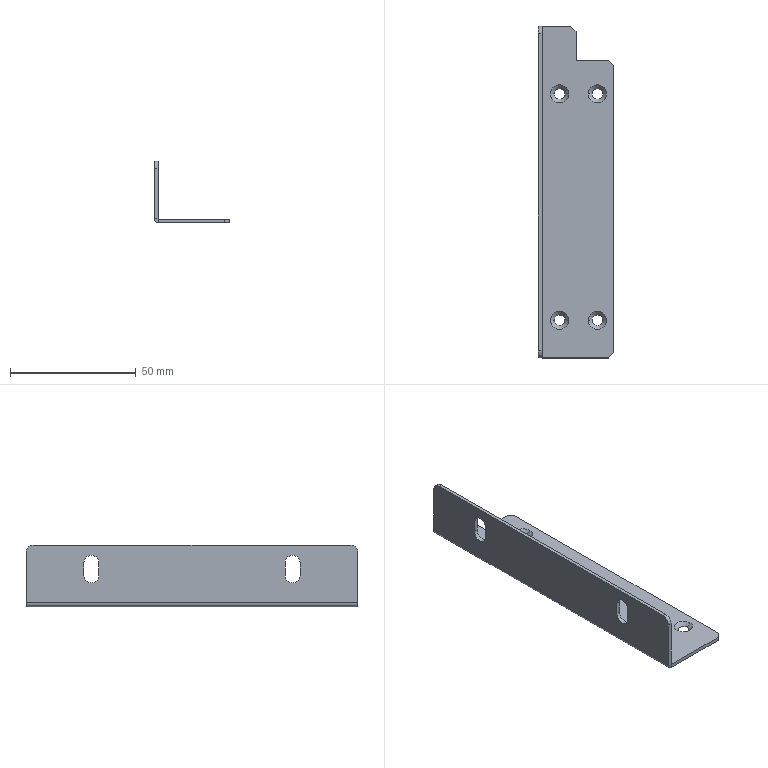Part | SolidWorks | features ICE 3, CornerTrim 2, Chamfer 1, EdgeFlange 1, FlatPattern 1, SMBaseFlange 1, SheetMetal 1 | 1 solid | 39 faces | box 30 x 132 x 24.5 mm | volume 9772 mm3 | plane 21 | cylinder 10 | cone 8 | commonest cylinder face diameters 6 x8 0.2 x1 3.2 x1
STEP:
#1=CARTESIAN_POINT('',(-8.6,39.,-1.5));
#2=VERTEX_POINT('',#1);
#3=CARTESIAN_POINT('',(-4.4,39.,-1.5));
#4=VERTEX_POINT('',#3);
#5=CARTESIAN_POINT('',(-6.5,39.,-1.5));
#6=DIRECTION('',(0.,0.,1.));
#7=DIRECTION('',(1.,0.,0.));
#8=AXIS2_PLACEMENT_3D('',#5,#6,#7);
#9=CIRCLE('',#8,2.1);
#10=EDGE_CURVE('',#2,#4,#9,.T.);
#11=ORIENTED_EDGE('',*,*,#10,.F.);
#12=CARTESIAN_POINT('',(-10.1,39.,0.));
#13=VERTEX_POINT('',#12);
#14=CARTESIAN_POINT('',(-8.6,39.,-1.5));
#15=DIRECTION('',(-0.7071,0.,0.7071));
#16=VECTOR('',#15,1000.);
#17=LINE('',#14,#16);
#18=EDGE_CURVE('',#2,#13,#17,.T.);
#19=ORIENTED_EDGE('',*,*,#18,.T.);
#20=CARTESIAN_POINT('',(-2.9,39.,0.));
#21=VERTEX_POINT('',#20);
#22=CARTESIAN_POINT('',(-6.5,39.,0.));
#23=DIRECTION('',(0.,0.,-1.));
#24=DIRECTION('',(1.,0.,0.));
#25=AXIS2_PLACEMENT_3D('',#22,#23,#24);
#26=CIRCLE('',#25,3.6);
#27=EDGE_CURVE('',#21,#13,#26,.T.);
#28=ORIENTED_EDGE('',*,*,#27,.F.);
#29=CARTESIAN_POINT('',(-4.4,39.,-1.5));
#30=DIRECTION('',(0.7071,0.,0.7071));
#31=VECTOR('',#30,1000.);
#32=LINE('',#29,#31);
#33=EDGE_CURVE('',#4,#21,#32,.T.);
#34=ORIENTED_EDGE('',*,*,#33,.F.);
#35=EDGE_LOOP('',(#11,#19,#28,#34));
#36=FACE_OUTER_BOUND('',#35,.T.);
#37=CARTESIAN_POINT('',(-6.5,39.,-1.5));
#38=DIRECTION('',(0.,0.,1.));
#39=DIRECTION('',(1.,0.,0.));
#40=AXIS2_PLACEMENT_3D('',#37,#38,#39);
#41=CONICAL_SURFACE('',#40,2.1,0.7854);
#42=ADVANCED_FACE('',(#36),#41,.F.);
#43=CARTESIAN_POINT('',(6.4,39.,-1.5));
#44=VERTEX_POINT('',#43);
#45=CARTESIAN_POINT('',(10.6,39.,-1.5));
#46=VERTEX_POINT('',#45);
#47=CARTESIAN_POINT('',(8.5,39.,-1.5));
#48=DIRECTION('',(0.,0.,1.));
#49=DIRECTION('',(1.,0.,0.));
#50=AXIS2_PLACEMENT_3D('',#47,#48,#49);
#51=CIRCLE('',#50,2.1);
#52=EDGE_CURVE('',#44,#46,#51,.T.);
#53=ORIENTED_EDGE('',*,*,#52,.F.);
#54=CARTESIAN_POINT('',(4.9,39.,0.));
#55=VERTEX_POINT('',#54);
#56=CARTESIAN_POINT('',(6.4,39.,-1.5));
#57=DIRECTION('',(-0.7071,0.,0.7071));
#58=VECTOR('',#57,1000.);
#59=LINE('',#56,#58);
#60=EDGE_CURVE('',#44,#55,#59,.T.);
#61=ORIENTED_EDGE('',*,*,#60,.T.);
#62=CARTESIAN_POINT('',(12.1,39.,0.));
#63=VERTEX_POINT('',#62);
#64=CARTESIAN_POINT('',(8.5,39.,0.));
#65=DIRECTION('',(0.,0.,-1.));
#66=DIRECTION('',(1.,0.,0.));
#67=AXIS2_PLACEMENT_3D('',#64,#65,#66);
#68=CIRCLE('',#67,3.6);
#69=EDGE_CURVE('',#63,#55,#68,.T.);
#70=ORIENTED_EDGE('',*,*,#69,.F.);
#71=CARTESIAN_POINT('',(10.6,39.,-1.5));
#72=DIRECTION('',(0.7071,0.,0.7071));
#73=VECTOR('',#72,1000.);
#74=LINE('',#71,#73);
#75=EDGE_CURVE('',#46,#63,#74,.T.);
#76=ORIENTED_EDGE('',*,*,#75,.F.);
#77=EDGE_LOOP('',(#53,#61,#70,#76));
#78=FACE_OUTER_BOUND('',#77,.T.);
#79=CARTESIAN_POINT('',(8.5,39.,-1.5));
#80=DIRECTION('',(0.,0.,1.));
#81=DIRECTION('',(1.,0.,0.));
#82=AXIS2_PLACEMENT_3D('',#79,#80,#81);
#83=CONICAL_SURFACE('',#82,2.1,0.7854);
#84=ADVANCED_FACE('',(#78),#83,.F.);
#85=CARTESIAN_POINT('',(6.4,-51.,-1.5));
#86=VERTEX_POINT('',#85);
#87=CARTESIAN_POINT('',(10.6,-51.,-1.5));
#88=VERTEX_POINT('',#87);
#89=CARTESIAN_POINT('',(8.5,-51.,-1.5));
#90=DIRECTION('',(0.,0.,1.));
#91=DIRECTION('',(1.,0.,0.));
#92=AXIS2_PLACEMENT_3D('',#89,#90,#91);
#93=CIRCLE('',#92,2.1);
#94=EDGE_CURVE('',#86,#88,#93,.T.);
#95=ORIENTED_EDGE('',*,*,#94,.F.);
#96=CARTESIAN_POINT('',(4.9,-51.,0.));
#97=VERTEX_POINT('',#96);
#98=CARTESIAN_POINT('',(6.4,-51.,-1.5));
#99=DIRECTION('',(-0.7071,0.,0.7071));
#100=VECTOR('',#99,1000.);
#101=LINE('',#98,#100);
#102=EDGE_CURVE('',#86,#97,#101,.T.);
#103=ORIENTED_EDGE('',*,*,#102,.T.);
#104=CARTESIAN_POINT('',(12.1,-51.,0.));
#105=VERTEX_POINT('',#104);
#106=CARTESIAN_POINT('',(8.5,-51.,0.));
#107=DIRECTION('',(0.,0.,-1.));
#108=DIRECTION('',(1.,0.,0.));
#109=AXIS2_PLACEMENT_3D('',#106,#107,#108);
#110=CIRCLE('',#109,3.6);
#111=EDGE_CURVE('',#105,#97,#110,.T.);
#112=ORIENTED_EDGE('',*,*,#111,.F.);
#113=CARTESIAN_POINT('',(10.6,-51.,-1.5));
#114=DIRECTION('',(0.7071,0.,0.7071));
#115=VECTOR('',#114,1000.);
#116=LINE('',#113,#115);
#117=EDGE_CURVE('',#88,#105,#116,.T.);
#118=ORIENTED_EDGE('',*,*,#117,.F.);
#119=EDGE_LOOP('',(#95,#103,#112,#118));
#120=FACE_OUTER_BOUND('',#119,.T.);
#121=CARTESIAN_POINT('',(8.5,-51.,-1.5));
#122=DIRECTION('',(0.,0.,1.));
#123=DIRECTION('',(1.,0.,0.));
#124=AXIS2_PLACEMENT_3D('',#121,#122,#123);
#125=CONICAL_SURFACE('',#124,2.1,0.7854);
#126=ADVANCED_FACE('',(#120),#125,.F.);
#127=CARTESIAN_POINT('',(-8.6,-51.,-1.5));
#128=VERTEX_POINT('',#127);
#129=CARTESIAN_POINT('',(-4.4,-51.,-1.5));
#130=VERTEX_POINT('',#129);
#131=CARTESIAN_POINT('',(-6.5,-51.,-1.5));
#132=DIRECTION('',(0.,0.,1.));
#133=DIRECTION('',(1.,0.,0.));
#134=AXIS2_PLACEMENT_3D('',#131,#132,#133);
#135=CIRCLE('',#134,2.1);
#136=EDGE_CURVE('',#128,#130,#135,.T.);
#137=ORIENTED_EDGE('',*,*,#136,.F.);
#138=CARTESIAN_POINT('',(-10.1,-51.,0.));
#139=VERTEX_POINT('',#138);
#140=CARTESIAN_POINT('',(-8.6,-51.,-1.5));
#141=DIRECTION('',(-0.7071,0.,0.7071));
#142=VECTOR('',#141,1000.);
#143=LINE('',#140,#142);
#144=EDGE_CURVE('',#128,#139,#143,.T.);
#145=ORIENTED_EDGE('',*,*,#144,.T.);
#146=CARTESIAN_POINT('',(-2.9,-51.,0.));
#147=VERTEX_POINT('',#146);
#148=CARTESIAN_POINT('',(-6.5,-51.,0.));
#149=DIRECTION('',(0.,0.,-1.));
#150=DIRECTION('',(1.,0.,0.));
#151=AXIS2_PLACEMENT_3D('',#148,#149,#150);
#152=CIRCLE('',#151,3.6);
#153=EDGE_CURVE('',#147,#139,#152,.T.);
#154=ORIENTED_EDGE('',*,*,#153,.F.);
#155=CARTESIAN_POINT('',(-4.4,-51.,-1.5));
#156=DIRECTION('',(0.7071,0.,0.7071));
#157=VECTOR('',#156,1000.);
#158=LINE('',#155,#157);
#159=EDGE_CURVE('',#130,#147,#158,.T.);
#160=ORIENTED_EDGE('',*,*,#159,.F.);
#161=EDGE_LOOP('',(#137,#145,#154,#160));
#162=FACE_OUTER_BOUND('',#161,.T.);
#163=CARTESIAN_POINT('',(-6.5,-51.,-1.5));
#164=DIRECTION('',(0.,0.,1.));
#165=DIRECTION('',(1.,0.,0.));
#166=AXIS2_PLACEMENT_3D('',#163,#164,#165);
#167=CONICAL_SURFACE('',#166,2.1,0.7854);
#168=ADVANCED_FACE('',(#162),#167,.F.);
#169=CARTESIAN_POINT('',(-13.5,43.,16.));
#170=VERTEX_POINT('',#169);
#171=CARTESIAN_POINT('',(-13.5,40.,19.));
#172=VERTEX_POINT('',#171);
#173=CARTESIAN_POINT('',(-13.5,40.,16.));
#174=DIRECTION('',(1.,0.,0.));
#175=DIRECTION('',(0.,0.,-1.));
#176=AXIS2_PLACEMENT_3D('',#173,#174,#175);
#177=CIRCLE('',#176,3.);
#178=EDGE_CURVE('',#170,#172,#177,.T.);
#179=ORIENTED_EDGE('',*,*,#178,.T.);
#180=CARTESIAN_POINT('',(-15.,40.,19.));
#181=VERTEX_POINT('',#180);
#182=CARTESIAN_POINT('',(-5.,40.,19.));
#183=DIRECTION('',(-1.,0.,0.));
#184=VECTOR('',#183,1000.);
#185=LINE('',#182,#184);
#186=EDGE_CURVE('',#172,#181,#185,.T.);
#187=ORIENTED_EDGE('',*,*,#186,.T.);
#188=CARTESIAN_POINT('',(-15.,43.,16.));
#189=VERTEX_POINT('',#188);
#190=CARTESIAN_POINT('',(-15.,40.,16.));
#191=DIRECTION('',(-1.,0.,0.));
#192=DIRECTION('',(0.,0.,1.));
#193=AXIS2_PLACEMENT_3D('',#190,#191,#192);
#194=CIRCLE('',#193,3.);
#195=EDGE_CURVE('',#181,#189,#194,.T.);
#196=ORIENTED_EDGE('',*,*,#195,.T.);
#197=CARTESIAN_POINT('',(-5.,43.,16.));
#198=DIRECTION('',(-1.,0.,0.));
#199=VECTOR('',#198,1000.);
#200=LINE('',#197,#199);
#201=EDGE_CURVE('',#170,#189,#200,.T.);
#202=ORIENTED_EDGE('',*,*,#201,.F.);
#203=EDGE_LOOP('',(#179,#187,#196,#202));
#204=FACE_OUTER_BOUND('',#203,.T.);
#205=CARTESIAN_POINT('',(-5.,40.,16.));
#206=DIRECTION('',(-1.,0.,0.));
#207=DIRECTION('',(0.,0.,1.));
#208=AXIS2_PLACEMENT_3D('',#205,#206,#207);
#209=CYLINDRICAL_SURFACE('',#208,3.);
#210=ADVANCED_FACE('',(#204),#209,.F.);
#211=CARTESIAN_POINT('',(-13.5,-37.,16.));
#212=VERTEX_POINT('',#211);
#213=CARTESIAN_POINT('',(-13.5,-40.,19.));
#214=VERTEX_POINT('',#213);
#215=CARTESIAN_POINT('',(-13.5,-40.,16.));
#216=DIRECTION('',(1.,0.,0.));
#217=DIRECTION('',(0.,0.,-1.));
#218=AXIS2_PLACEMENT_3D('',#215,#216,#217);
#219=CIRCLE('',#218,3.);
#220=EDGE_CURVE('',#212,#214,#219,.T.);
#221=ORIENTED_EDGE('',*,*,#220,.T.);
#222=CARTESIAN_POINT('',(-15.,-40.,19.));
#223=VERTEX_POINT('',#222);
#224=CARTESIAN_POINT('',(-5.,-40.,19.));
#225=DIRECTION('',(-1.,0.,0.));
#226=VECTOR('',#225,1000.);
#227=LINE('',#224,#226);
#228=EDGE_CURVE('',#214,#223,#227,.T.);
#229=ORIENTED_EDGE('',*,*,#228,.T.);
#230=CARTESIAN_POINT('',(-15.,-37.,16.));
#231=VERTEX_POINT('',#230);
#232=CARTESIAN_POINT('',(-15.,-40.,16.));
#233=DIRECTION('',(-1.,0.,0.));
#234=DIRECTION('',(0.,0.,1.));
#235=AXIS2_PLACEMENT_3D('',#232,#233,#234);
#236=CIRCLE('',#235,3.);
#237=EDGE_CURVE('',#223,#231,#236,.T.);
#238=ORIENTED_EDGE('',*,*,#237,.T.);
#239=CARTESIAN_POINT('',(-5.,-37.,16.));
#240=DIRECTION('',(-1.,0.,0.));
#241=VECTOR('',#240,1000.);
#242=LINE('',#239,#241);
#243=EDGE_CURVE('',#212,#231,#242,.T.);
#244=ORIENTED_EDGE('',*,*,#243,.F.);
#245=EDGE_LOOP('',(#221,#229,#238,#244));
#246=FACE_OUTER_BOUND('',#245,.T.);
#247=CARTESIAN_POINT('',(-5.,-40.,16.));
#248=DIRECTION('',(-1.,0.,0.));
#249=DIRECTION('',(0.,0.,1.));
#250=AXIS2_PLACEMENT_3D('',#247,#248,#249);
#251=CYLINDRICAL_SURFACE('',#250,3.);
#252=ADVANCED_FACE('',(#246),#251,.F.);
#253=CARTESIAN_POINT('',(-13.4,-66.,-1.5));
#254=VERTEX_POINT('',#253);
#255=CARTESIAN_POINT('',(13.,-66.,-1.5));
#256=VERTEX_POINT('',#255);
#257=CARTESIAN_POINT('',(-15.,-66.,-1.5));
#258=DIRECTION('',(1.,0.,0.));
#259=VECTOR('',#258,1000.);
#260=LINE('',#257,#259);
#261=EDGE_CURVE('',#254,#256,#260,.T.);
#262=ORIENTED_EDGE('',*,*,#261,.T.);
#263=CARTESIAN_POINT('',(13.,-66.,0.));
#264=VERTEX_POINT('',#263);
#265=CARTESIAN_POINT('',(13.,-66.,-1.5));
#266=DIRECTION('',(0.,0.,1.));
#267=VECTOR('',#266,1000.);
#268=LINE('',#265,#267);
#269=EDGE_CURVE('',#256,#264,#268,.T.);
#270=ORIENTED_EDGE('',*,*,#269,.T.);
#271=CARTESIAN_POINT('',(-13.4,-66.,0.));
#272=VERTEX_POINT('',#271);
#273=CARTESIAN_POINT('',(-15.,-66.,0.));
#274=DIRECTION('',(1.,0.,0.));
#275=VECTOR('',#274,1000.);
#276=LINE('',#273,#275);
#277=EDGE_CURVE('',#272,#264,#276,.T.);
#278=ORIENTED_EDGE('',*,*,#277,.F.);
#279=CARTESIAN_POINT('',(-13.4,-66.,0.));
#280=DIRECTION('',(0.,0.,-1.));
#281=VECTOR('',#280,1000.);
#282=LINE('',#279,#281);
#283=EDGE_CURVE('',#272,#254,#282,.T.);
#284=ORIENTED_EDGE('',*,*,#283,.T.);
#285=EDGE_LOOP('',(#262,#270,#278,#284));
#286=FACE_OUTER_BOUND('',#285,.T.);
#287=CARTESIAN_POINT('',(-15.,-66.,-1.5));
#288=DIRECTION('',(0.,-1.,0.));
#289=DIRECTION('',(0.,0.,-1.));
#290=AXIS2_PLACEMENT_3D('',#287,#288,#289);
#291=PLANE('',#290);
#292=ADVANCED_FACE('',(#286),#291,.T.);
#293=CARTESIAN_POINT('',(-6.5,-51.,-1.5));
#294=DIRECTION('',(0.,0.,1.));
#295=DIRECTION('',(1.,0.,0.));
#296=AXIS2_PLACEMENT_3D('',#293,#294,#295);
#297=CIRCLE('',#296,2.1);
#298=EDGE_CURVE('',#130,#128,#297,.T.);
#299=ORIENTED_EDGE('',*,*,#298,.T.);
#300=ORIENTED_EDGE('',*,*,#136,.T.);
#301=EDGE_LOOP('',(#299,#300));
#302=FACE_BOUND('',#301,.T.);
#303=CARTESIAN_POINT('',(8.5,-51.,-1.5));
#304=DIRECTION('',(0.,0.,1.));
#305=DIRECTION('',(1.,0.,0.));
#306=AXIS2_PLACEMENT_3D('',#303,#304,#305);
#307=CIRCLE('',#306,2.1);
#308=EDGE_CURVE('',#88,#86,#307,.T.);
#309=ORIENTED_EDGE('',*,*,#308,.T.);
#310=ORIENTED_EDGE('',*,*,#94,.T.);
#311=EDGE_LOOP('',(#309,#310));
#312=FACE_BOUND('',#311,.T.);
#313=CARTESIAN_POINT('',(8.5,39.,-1.5));
#314=DIRECTION('',(0.,0.,1.));
#315=DIRECTION('',(1.,0.,0.));
#316=AXIS2_PLACEMENT_3D('',#313,#314,#315);
#317=CIRCLE('',#316,2.1);
#318=EDGE_CURVE('',#46,#44,#317,.T.);
#319=ORIENTED_EDGE('',*,*,#318,.T.);
#320=ORIENTED_EDGE('',*,*,#52,.T.);
#321=EDGE_LOOP('',(#319,#320));
#322=FACE_BOUND('',#321,.T.);
#323=CARTESIAN_POINT('',(-6.5,39.,-1.5));
#324=DIRECTION('',(0.,0.,1.));
#325=DIRECTION('',(1.,0.,0.));
#326=AXIS2_PLACEMENT_3D('',#323,#324,#325);
#327=CIRCLE('',#326,2.1);
#328=EDGE_CURVE('',#4,#2,#327,.T.);
#329=ORIENTED_EDGE('',*,*,#328,.T.);
#330=ORIENTED_EDGE('',*,*,#10,.T.);
#331=EDGE_LOOP('',(#329,#330));
#332=FACE_BOUND('',#331,.T.);
#333=CARTESIAN_POINT('',(0.,52.5,-1.5));
#334=VERTEX_POINT('',#333);
#335=CARTESIAN_POINT('',(13.,52.5,-1.5));
#336=VERTEX_POINT('',#335);
#337=CARTESIAN_POINT('',(0.,52.5,-1.5));
#338=DIRECTION('',(1.,0.,0.));
#339=VECTOR('',#338,1000.);
#340=LINE('',#337,#339);
#341=EDGE_CURVE('',#334,#336,#340,.T.);
#342=ORIENTED_EDGE('',*,*,#341,.T.);
#343=CARTESIAN_POINT('',(15.,50.5,-1.5));
#344=VERTEX_POINT('',#343);
#345=CARTESIAN_POINT('',(15.,50.5,-1.5));
#346=DIRECTION('',(0.7071,-0.7071,0.));
#347=VECTOR('',#346,1000.);
#348=LINE('',#345,#347);
#349=EDGE_CURVE('',#336,#344,#348,.T.);
#350=ORIENTED_EDGE('',*,*,#349,.T.);
#351=CARTESIAN_POINT('',(15.,-64.,-1.5));
#352=VERTEX_POINT('',#351);
#353=CARTESIAN_POINT('',(15.,66.,-1.5));
#354=DIRECTION('',(0.,1.,0.));
#355=VECTOR('',#354,1000.);
#356=LINE('',#353,#355);
#357=EDGE_CURVE('',#352,#344,#356,.T.);
#358=ORIENTED_EDGE('',*,*,#357,.F.);
#359=CARTESIAN_POINT('',(13.,-66.,-1.5));
#360=DIRECTION('',(-0.7071,-0.7071,0.));
#361=VECTOR('',#360,1000.);
#362=LINE('',#359,#361);
#363=EDGE_CURVE('',#352,#256,#362,.T.);
#364=ORIENTED_EDGE('',*,*,#363,.T.);
#365=ORIENTED_EDGE('',*,*,#261,.F.);
#366=CARTESIAN_POINT('',(-13.4,66.,-1.5));
#367=VERTEX_POINT('',#366);
#368=CARTESIAN_POINT('',(-13.4,-66.,-1.5));
#369=DIRECTION('',(0.,1.,0.));
#370=VECTOR('',#369,1000.);
#371=LINE('',#368,#370);
#372=EDGE_CURVE('',#254,#367,#371,.T.);
#373=ORIENTED_EDGE('',*,*,#372,.T.);
#374=CARTESIAN_POINT('',(-2.,66.,-1.5));
#375=VERTEX_POINT('',#374);
#376=CARTESIAN_POINT('',(-15.,66.,-1.5));
#377=DIRECTION('',(-1.,0.,0.));
#378=VECTOR('',#377,1000.);
#379=LINE('',#376,#378);
#380=EDGE_CURVE('',#375,#367,#379,.T.);
#381=ORIENTED_EDGE('',*,*,#380,.F.);
#382=CARTESIAN_POINT('',(0.,64.,-1.5));
#383=VERTEX_POINT('',#382);
#384=CARTESIAN_POINT('',(0.,64.,-1.5));
#385=DIRECTION('',(0.7071,-0.7071,0.));
#386=VECTOR('',#385,1000.);
#387=LINE('',#384,#386);
#388=EDGE_CURVE('',#375,#383,#387,.T.);
#389=ORIENTED_EDGE('',*,*,#388,.T.);
#390=CARTESIAN_POINT('',(0.,0.,-1.5));
#391=DIRECTION('',(0.,-1.,0.));
#392=VECTOR('',#391,1000.);
#393=LINE('',#390,#392);
#394=EDGE_CURVE('',#383,#334,#393,.T.);
#395=ORIENTED_EDGE('',*,*,#394,.T.);
#396=EDGE_LOOP('',(#342,#350,#358,#364,#365,#373,#381,#389,#395));
#397=FACE_OUTER_BOUND('',#396,.T.);
#398=CARTESIAN_POINT('',(0.,0.,-1.5));
#399=DIRECTION('',(0.,0.,1.));
#400=DIRECTION('',(1.,0.,0.));
#401=AXIS2_PLACEMENT_3D('',#398,#399,#400);
#402=PLANE('',#401);
#403=ADVANCED_FACE('',(#302,#312,#322,#332,#397),#402,.F.);
#404=ORIENTED_EDGE('',*,*,#153,.T.);
#405=CARTESIAN_POINT('',(-6.5,-51.,0.));
#406=DIRECTION('',(0.,0.,-1.));
#407=DIRECTION('',(1.,0.,0.));
#408=AXIS2_PLACEMENT_3D('',#405,#406,#407);
#409=CIRCLE('',#408,3.6);
#410=EDGE_CURVE('',#139,#147,#409,.T.);
#411=ORIENTED_EDGE('',*,*,#410,.T.);
#412=EDGE_LOOP('',(#404,#411));
#413=FACE_BOUND('',#412,.T.);
#414=ORIENTED_EDGE('',*,*,#111,.T.);
#415=CARTESIAN_POINT('',(8.5,-51.,0.));
#416=DIRECTION('',(0.,0.,-1.));
#417=DIRECTION('',(1.,0.,0.));
#418=AXIS2_PLACEMENT_3D('',#415,#416,#417);
#419=CIRCLE('',#418,3.6);
#420=EDGE_CURVE('',#97,#105,#419,.T.);
#421=ORIENTED_EDGE('',*,*,#420,.T.);
#422=EDGE_LOOP('',(#414,#421));
#423=FACE_BOUND('',#422,.T.);
#424=ORIENTED_EDGE('',*,*,#69,.T.);
#425=CARTESIAN_POINT('',(8.5,39.,0.));
#426=DIRECTION('',(0.,0.,-1.));
#427=DIRECTION('',(1.,0.,0.));
#428=AXIS2_PLACEMENT_3D('',#425,#426,#427);
#429=CIRCLE('',#428,3.6);
#430=EDGE_CURVE('',#55,#63,#429,.T.);
#431=ORIENTED_EDGE('',*,*,#430,.T.);
#432=EDGE_LOOP('',(#424,#431));
#433=FACE_BOUND('',#432,.T.);
#434=ORIENTED_EDGE('',*,*,#27,.T.);
#435=CARTESIAN_POINT('',(-6.5,39.,0.));
#436=DIRECTION('',(0.,0.,-1.));
#437=DIRECTION('',(1.,0.,0.));
#438=AXIS2_PLACEMENT_3D('',#435,#436,#437);
#439=CIRCLE('',#438,3.6);
#440=EDGE_CURVE('',#13,#21,#439,.T.);
#441=ORIENTED_EDGE('',*,*,#440,.T.);
#442=EDGE_LOOP('',(#434,#441));
#443=FACE_BOUND('',#442,.T.);
#444=CARTESIAN_POINT('',(15.,-64.,0.));
#445=VERTEX_POINT('',#444);
#446=CARTESIAN_POINT('',(15.,50.5,0.));
#447=VERTEX_POINT('',#446);
#448=CARTESIAN_POINT('',(15.,66.,0.));
#449=DIRECTION('',(0.,1.,0.));
#450=VECTOR('',#449,1000.);
#451=LINE('',#448,#450);
#452=EDGE_CURVE('',#445,#447,#451,.T.);
#453=ORIENTED_EDGE('',*,*,#452,.T.);
#454=CARTESIAN_POINT('',(13.,52.5,0.));
#455=VERTEX_POINT('',#454);
#456=CARTESIAN_POINT('',(32.75,32.75,0.));
#457=DIRECTION('',(-0.7071,0.7071,0.));
#458=VECTOR('',#457,1000.);
#459=LINE('',#456,#458);
#460=EDGE_CURVE('',#447,#455,#459,.T.);
#461=ORIENTED_EDGE('',*,*,#460,.T.);
#462=CARTESIAN_POINT('',(0.,52.5,0.));
#463=VERTEX_POINT('',#462);
#464=CARTESIAN_POINT('',(15.,52.5,0.));
#465=DIRECTION('',(1.,0.,0.));
#466=VECTOR('',#465,1000.);
#467=LINE('',#464,#466);
#468=EDGE_CURVE('',#463,#455,#467,.T.);
#469=ORIENTED_EDGE('',*,*,#468,.F.);
#470=CARTESIAN_POINT('',(0.,64.,0.));
#471=VERTEX_POINT('',#470);
#472=CARTESIAN_POINT('',(0.,66.,0.));
#473=DIRECTION('',(0.,-1.,0.));
#474=VECTOR('',#473,1000.);
#475=LINE('',#472,#474);
#476=EDGE_CURVE('',#471,#463,#475,.T.);
#477=ORIENTED_EDGE('',*,*,#476,.F.);
#478=CARTESIAN_POINT('',(-2.,66.,0.));
#479=VERTEX_POINT('',#478);
#480=CARTESIAN_POINT('',(32.,32.,0.));
#481=DIRECTION('',(-0.7071,0.7071,0.));
#482=VECTOR('',#481,1000.);
#483=LINE('',#480,#482);
#484=EDGE_CURVE('',#471,#479,#483,.T.);
#485=ORIENTED_EDGE('',*,*,#484,.T.);
#486=CARTESIAN_POINT('',(-13.4,66.,0.));
#487=VERTEX_POINT('',#486);
#488=CARTESIAN_POINT('',(-15.,66.,0.));
#489=DIRECTION('',(-1.,0.,0.));
#490=VECTOR('',#489,1000.);
#491=LINE('',#488,#490);
#492=EDGE_CURVE('',#479,#487,#491,.T.);
#493=ORIENTED_EDGE('',*,*,#492,.T.);
#494=CARTESIAN_POINT('',(-13.4,-66.,0.));
#495=DIRECTION('',(0.,1.,0.));
#496=VECTOR('',#495,1000.);
#497=LINE('',#494,#496);
#498=EDGE_CURVE('',#272,#487,#497,.T.);
#499=ORIENTED_EDGE('',*,*,#498,.F.);
#500=ORIENTED_EDGE('',*,*,#277,.T.);
#501=CARTESIAN_POINT('',(39.5,-39.5,0.));
#502=DIRECTION('',(0.7071,0.7071,0.));
#503=VECTOR('',#502,1000.);
#504=LINE('',#501,#503);
#505=EDGE_CURVE('',#264,#445,#504,.T.);
#506=ORIENTED_EDGE('',*,*,#505,.T.);
#507=EDGE_LOOP('',(#453,#461,#469,#477,#485,#493,#499,#500,#506));
#508=FACE_OUTER_BOUND('',#507,.T.);
#509=CARTESIAN_POINT('',(0.,0.,0.));
#510=DIRECTION('',(0.,0.,1.));
#511=DIRECTION('',(1.,0.,0.));
#512=AXIS2_PLACEMENT_3D('',#509,#510,#511);
#513=PLANE('',#512);
#514=ADVANCED_FACE('',(#413,#423,#433,#443,#508),#513,.T.);
#515=ORIENTED_EDGE('',*,*,#357,.T.);
#516=CARTESIAN_POINT('',(15.,50.5,0.));
#517=DIRECTION('',(0.,0.,1.));
#518=VECTOR('',#517,1000.);
#519=LINE('',#516,#518);
#520=EDGE_CURVE('',#344,#447,#519,.T.);
#521=ORIENTED_EDGE('',*,*,#520,.T.);
#522=ORIENTED_EDGE('',*,*,#452,.F.);
#523=CARTESIAN_POINT('',(15.,-64.,-1.5));
#524=DIRECTION('',(0.,0.,-1.));
#525=VECTOR('',#524,1000.);
#526=LINE('',#523,#525);
#527=EDGE_CURVE('',#445,#352,#526,.T.);
#528=ORIENTED_EDGE('',*,*,#527,.T.);
#529=EDGE_LOOP('',(#515,#521,#522,#528));
#530=FACE_OUTER_BOUND('',#529,.T.);
#531=CARTESIAN_POINT('',(15.,66.,-1.5));
#532=DIRECTION('',(1.,0.,0.));
#533=DIRECTION('',(0.,1.,0.));
#534=AXIS2_PLACEMENT_3D('',#531,#532,#533);
#535=PLANE('',#534);
#536=ADVANCED_FACE('',(#530),#535,.T.);
#537=ORIENTED_EDGE('',*,*,#492,.F.);
#538=CARTESIAN_POINT('',(-2.,66.,-1.5));
#539=DIRECTION('',(0.,0.,-1.));
#540=VECTOR('',#539,1000.);
#541=LINE('',#538,#540);
#542=EDGE_CURVE('',#479,#375,#541,.T.);
#543=ORIENTED_EDGE('',*,*,#542,.T.);
#544=ORIENTED_EDGE('',*,*,#380,.T.);
#545=CARTESIAN_POINT('',(-13.4,66.,0.));
#546=DIRECTION('',(0.,0.,-1.));
#547=VECTOR('',#546,1000.);
#548=LINE('',#545,#547);
#549=EDGE_CURVE('',#487,#367,#548,.T.);
#550=ORIENTED_EDGE('',*,*,#549,.F.);
#551=EDGE_LOOP('',(#537,#543,#544,#550));
#552=FACE_OUTER_BOUND('',#551,.T.);
#553=CARTESIAN_POINT('',(-15.,66.,-1.5));
#554=DIRECTION('',(0.,1.,0.));
#555=DIRECTION('',(0.,0.,1.));
#556=AXIS2_PLACEMENT_3D('',#553,#554,#555);
#557=PLANE('',#556);
#558=ADVANCED_FACE('',(#552),#557,.T.);
#559=CARTESIAN_POINT('',(-13.5,66.,0.1));
#560=VERTEX_POINT('',#559);
#561=CARTESIAN_POINT('',(-15.,66.,0.1));
#562=VERTEX_POINT('',#561);
#563=CARTESIAN_POINT('',(-15.,66.,0.1));
#564=DIRECTION('',(-1.,0.,0.));
#565=VECTOR('',#564,1000.);
#566=LINE('',#563,#565);
#567=EDGE_CURVE('',#560,#562,#566,.T.);
#568=ORIENTED_EDGE('',*,*,#567,.F.);
#569=CARTESIAN_POINT('',(-13.4,66.,0.1));
#570=DIRECTION('',(0.,1.,0.));
#571=DIRECTION('',(0.,0.,-1.));
#572=AXIS2_PLACEMENT_3D('',#569,#570,#571);
#573=CIRCLE('',#572,0.1);
#574=EDGE_CURVE('',#487,#560,#573,.T.);
#575=ORIENTED_EDGE('',*,*,#574,.F.);
#576=ORIENTED_EDGE('',*,*,#549,.T.);
#577=CARTESIAN_POINT('',(-13.4,66.,0.1));
#578=DIRECTION('',(0.,1.,0.));
#579=DIRECTION('',(0.,0.,-1.));
#580=AXIS2_PLACEMENT_3D('',#577,#578,#579);
#581=CIRCLE('',#580,1.6);
#582=EDGE_CURVE('',#367,#562,#581,.T.);
#583=ORIENTED_EDGE('',*,*,#582,.T.);
#584=EDGE_LOOP('',(#568,#575,#576,#583));
#585=FACE_OUTER_BOUND('',#584,.T.);
#586=CARTESIAN_POINT('',(-13.4,66.,0.1));
#587=DIRECTION('',(0.,1.,0.));
#588=DIRECTION('',(0.,0.,1.));
#589=AXIS2_PLACEMENT_3D('',#586,#587,#588);
#590=PLANE('',#589);
#591=ADVANCED_FACE('',(#585),#590,.T.);
#592=CARTESIAN_POINT('',(-13.5,-66.,0.1));
#593=VERTEX_POINT('',#592);
#594=CARTESIAN_POINT('',(-13.4,-66.,0.1));
#595=DIRECTION('',(0.,-1.,0.));
#596=DIRECTION('',(0.,0.,-1.));
#597=AXIS2_PLACEMENT_3D('',#594,#595,#596);
#598=CIRCLE('',#597,0.1);
#599=EDGE_CURVE('',#593,#272,#598,.T.);
#600=ORIENTED_EDGE('',*,*,#599,.F.);
#601=CARTESIAN_POINT('',(-15.,-66.,0.1));
#602=VERTEX_POINT('',#601);
#603=CARTESIAN_POINT('',(-13.5,-66.,0.1));
#604=DIRECTION('',(-1.,0.,0.));
#605=VECTOR('',#604,1000.);
#606=LINE('',#603,#605);
#607=EDGE_CURVE('',#593,#602,#606,.T.);
#608=ORIENTED_EDGE('',*,*,#607,.T.);
#609=CARTESIAN_POINT('',(-13.4,-66.,0.1));
#610=DIRECTION('',(0.,-1.,0.));
#611=DIRECTION('',(0.,0.,-1.));
#612=AXIS2_PLACEMENT_3D('',#609,#610,#611);
#613=CIRCLE('',#612,1.6);
#614=EDGE_CURVE('',#602,#254,#613,.T.);
#615=ORIENTED_EDGE('',*,*,#614,.T.);
#616=ORIENTED_EDGE('',*,*,#283,.F.);
#617=EDGE_LOOP('',(#600,#608,#615,#616));
#618=FACE_OUTER_BOUND('',#617,.T.);
#619=CARTESIAN_POINT('',(-13.4,-66.,0.1));
#620=DIRECTION('',(0.,1.,0.));
#621=DIRECTION('',(0.,0.,1.));
#622=AXIS2_PLACEMENT_3D('',#619,#620,#621);
#623=PLANE('',#622);
#624=ADVANCED_FACE('',(#618),#623,.F.);
#625=ORIENTED_EDGE('',*,*,#372,.F.);
#626=ORIENTED_EDGE('',*,*,#614,.F.);
#627=CARTESIAN_POINT('',(-15.,66.,0.1));
#628=DIRECTION('',(0.,1.,0.));
#629=VECTOR('',#628,1000.);
#630=LINE('',#627,#629);
#631=EDGE_CURVE('',#602,#562,#630,.T.);
#632=ORIENTED_EDGE('',*,*,#631,.T.);
#633=ORIENTED_EDGE('',*,*,#582,.F.);
#634=EDGE_LOOP('',(#625,#626,#632,#633));
#635=FACE_OUTER_BOUND('',#634,.T.);
#636=CARTESIAN_POINT('',(-13.4,-66.,0.1));
#637=DIRECTION('',(0.,-1.,0.));
#638=DIRECTION('',(-1.,0.,0.));
#639=AXIS2_PLACEMENT_3D('',#636,#637,#638);
#640=CYLINDRICAL_SURFACE('',#639,1.6);
#641=ADVANCED_FACE('',(#635),#640,.T.);
#642=ORIENTED_EDGE('',*,*,#498,.T.);
#643=ORIENTED_EDGE('',*,*,#574,.T.);
#644=CARTESIAN_POINT('',(-13.5,66.,0.1));
#645=DIRECTION('',(0.,-1.,0.));
#646=VECTOR('',#645,1000.);
#647=LINE('',#644,#646);
#648=EDGE_CURVE('',#560,#593,#647,.T.);
#649=ORIENTED_EDGE('',*,*,#648,.T.);
#650=ORIENTED_EDGE('',*,*,#599,.T.);
#651=EDGE_LOOP('',(#642,#643,#649,#650));
#652=FACE_OUTER_BOUND('',#651,.T.);
#653=CARTESIAN_POINT('',(-13.4,-66.,0.1));
#654=DIRECTION('',(0.,-1.,0.));
#655=DIRECTION('',(-1.,0.,0.));
#656=AXIS2_PLACEMENT_3D('',#653,#654,#655);
#657=CYLINDRICAL_SURFACE('',#656,0.1);
#658=ADVANCED_FACE('',(#652),#657,.F.);
#659=CARTESIAN_POINT('',(-15.,66.,20.));
#660=VERTEX_POINT('',#659);
#661=CARTESIAN_POINT('',(-15.,66.,0.));
#662=DIRECTION('',(0.,0.,-1.));
#663=VECTOR('',#662,1000.);
#664=LINE('',#661,#663);
#665=EDGE_CURVE('',#660,#562,#664,.T.);
#666=ORIENTED_EDGE('',*,*,#665,.F.);
#667=CARTESIAN_POINT('',(-13.5,66.,20.));
#668=VERTEX_POINT('',#667);
#669=CARTESIAN_POINT('',(-15.,66.,20.));
#670=DIRECTION('',(1.,0.,0.));
#671=VECTOR('',#670,1000.);
#672=LINE('',#669,#671);
#673=EDGE_CURVE('',#660,#668,#672,.T.);
#674=ORIENTED_EDGE('',*,*,#673,.T.);
#675=CARTESIAN_POINT('',(-13.5,66.,0.));
#676=DIRECTION('',(0.,0.,-1.));
#677=VECTOR('',#676,1000.);
#678=LINE('',#675,#677);
#679=EDGE_CURVE('',#668,#560,#678,.T.);
#680=ORIENTED_EDGE('',*,*,#679,.T.);
#681=ORIENTED_EDGE('',*,*,#567,.T.);
#682=EDGE_LOOP('',(#666,#674,#680,#681));
#683=FACE_OUTER_BOUND('',#682,.T.);
#684=CARTESIAN_POINT('',(-15.,66.,0.));
#685=DIRECTION('',(0.,-1.,0.));
#686=DIRECTION('',(1.,0.,0.));
#687=AXIS2_PLACEMENT_3D('',#684,#685,#686);
#688=PLANE('',#687);
#689=ADVANCED_FACE('',(#683),#688,.F.);
#690=CARTESIAN_POINT('',(-13.5,-66.,20.));
#691=VERTEX_POINT('',#690);
#692=CARTESIAN_POINT('',(-13.5,-66.,23.));
#693=DIRECTION('',(0.,0.,1.));
#694=VECTOR('',#693,1000.);
#695=LINE('',#692,#694);
#696=EDGE_CURVE('',#593,#691,#695,.T.);
#697=ORIENTED_EDGE('',*,*,#696,.T.);
#698=CARTESIAN_POINT('',(-15.,-66.,20.));
#699=VERTEX_POINT('',#698);
#700=CARTESIAN_POINT('',(-15.,-66.,20.));
#701=DIRECTION('',(-1.,0.,0.));
#702=VECTOR('',#701,1000.);
#703=LINE('',#700,#702);
#704=EDGE_CURVE('',#691,#699,#703,.T.);
#705=ORIENTED_EDGE('',*,*,#704,.T.);
#706=CARTESIAN_POINT('',(-15.,-66.,0.));
#707=DIRECTION('',(0.,0.,1.));
#708=VECTOR('',#707,1000.);
#709=LINE('',#706,#708);
#710=EDGE_CURVE('',#602,#699,#709,.T.);
#711=ORIENTED_EDGE('',*,*,#710,.F.);
#712=ORIENTED_EDGE('',*,*,#607,.F.);
#713=EDGE_LOOP('',(#697,#705,#711,#712));
#714=FACE_OUTER_BOUND('',#713,.T.);
#715=CARTESIAN_POINT('',(-15.,-66.,23.));
#716=DIRECTION('',(0.,1.,0.));
#717=DIRECTION('',(-1.,0.,0.));
#718=AXIS2_PLACEMENT_3D('',#715,#716,#717);
#719=PLANE('',#718);
#720=ADVANCED_FACE('',(#714),#719,.F.);
#721=CARTESIAN_POINT('',(-15.,37.,11.));
#722=VERTEX_POINT('',#721);
#723=CARTESIAN_POINT('',(-15.,37.,16.));
#724=VERTEX_POINT('',#723);
#725=CARTESIAN_POINT('',(-15.,37.,11.));
#726=DIRECTION('',(0.,0.,1.));
#727=VECTOR('',#726,1000.);
#728=LINE('',#725,#727);
#729=EDGE_CURVE('',#722,#724,#728,.T.);
#730=ORIENTED_EDGE('',*,*,#729,.F.);
#731=CARTESIAN_POINT('',(-15.,43.,11.));
#732=VERTEX_POINT('',#731);
#733=CARTESIAN_POINT('',(-15.,40.,11.));
#734=DIRECTION('',(-1.,0.,0.));
#735=DIRECTION('',(0.,0.,1.));
#736=AXIS2_PLACEMENT_3D('',#733,#734,#735);
#737=CIRCLE('',#736,3.);
#738=EDGE_CURVE('',#732,#722,#737,.T.);
#739=ORIENTED_EDGE('',*,*,#738,.F.);
#740=CARTESIAN_POINT('',(-15.,43.,11.));
#741=DIRECTION('',(0.,0.,-1.));
#742=VECTOR('',#741,1000.);
#743=LINE('',#740,#742);
#744=EDGE_CURVE('',#189,#732,#743,.T.);
#745=ORIENTED_EDGE('',*,*,#744,.F.);
#746=ORIENTED_EDGE('',*,*,#195,.F.);
#747=CARTESIAN_POINT('',(-15.,40.,16.));
#748=DIRECTION('',(-1.,0.,0.));
#749=DIRECTION('',(0.,0.,1.));
#750=AXIS2_PLACEMENT_3D('',#747,#748,#749);
#751=CIRCLE('',#750,3.);
#752=EDGE_CURVE('',#724,#181,#751,.T.);
#753=ORIENTED_EDGE('',*,*,#752,.F.);
#754=EDGE_LOOP('',(#730,#739,#745,#746,#753));
#755=FACE_BOUND('',#754,.T.);
#756=CARTESIAN_POINT('',(-15.,-43.,11.));
#757=VERTEX_POINT('',#756);
#758=CARTESIAN_POINT('',(-15.,-43.,16.));
#759=VERTEX_POINT('',#758);
#760=CARTESIAN_POINT('',(-15.,-43.,11.));
#761=DIRECTION('',(0.,0.,1.));
#762=VECTOR('',#761,1000.);
#763=LINE('',#760,#762);
#764=EDGE_CURVE('',#757,#759,#763,.T.);
#765=ORIENTED_EDGE('',*,*,#764,.F.);
#766=CARTESIAN_POINT('',(-15.,-37.,11.));
#767=VERTEX_POINT('',#766);
#768=CARTESIAN_POINT('',(-15.,-40.,11.));
#769=DIRECTION('',(-1.,0.,0.));
#770=DIRECTION('',(0.,0.,1.));
#771=AXIS2_PLACEMENT_3D('',#768,#769,#770);
#772=CIRCLE('',#771,3.);
#773=EDGE_CURVE('',#767,#757,#772,.T.);
#774=ORIENTED_EDGE('',*,*,#773,.F.);
#775=CARTESIAN_POINT('',(-15.,-37.,11.));
#776=DIRECTION('',(0.,0.,-1.));
#777=VECTOR('',#776,1000.);
#778=LINE('',#775,#777);
#779=EDGE_CURVE('',#231,#767,#778,.T.);
#780=ORIENTED_EDGE('',*,*,#779,.F.);
#781=ORIENTED_EDGE('',*,*,#237,.F.);
#782=CARTESIAN_POINT('',(-15.,-40.,16.));
#783=DIRECTION('',(-1.,0.,0.));
#784=DIRECTION('',(0.,0.,1.));
#785=AXIS2_PLACEMENT_3D('',#782,#783,#784);
#786=CIRCLE('',#785,3.);
#787=EDGE_CURVE('',#759,#223,#786,.T.);
#788=ORIENTED_EDGE('',*,*,#787,.F.);
#789=EDGE_LOOP('',(#765,#774,#780,#781,#788));
#790=FACE_BOUND('',#789,.T.);
#791=CARTESIAN_POINT('',(-15.,-63.,23.));
#792=VERTEX_POINT('',#791);
#793=CARTESIAN_POINT('',(-15.,63.,23.));
#794=VERTEX_POINT('',#793);
#795=CARTESIAN_POINT('',(-15.,0.,23.));
#796=DIRECTION('',(0.,1.,0.));
#797=VECTOR('',#796,1000.);
#798=LINE('',#795,#797);
#799=EDGE_CURVE('',#792,#794,#798,.T.);
#800=ORIENTED_EDGE('',*,*,#799,.T.);
#801=CARTESIAN_POINT('',(-15.,63.,20.));
#802=DIRECTION('',(-1.,0.,0.));
#803=DIRECTION('',(0.,0.,-1.));
#804=AXIS2_PLACEMENT_3D('',#801,#802,#803);
#805=CIRCLE('',#804,3.);
#806=EDGE_CURVE('',#794,#660,#805,.T.);
#807=ORIENTED_EDGE('',*,*,#806,.T.);
#808=ORIENTED_EDGE('',*,*,#665,.T.);
#809=ORIENTED_EDGE('',*,*,#631,.F.);
#810=ORIENTED_EDGE('',*,*,#710,.T.);
#811=CARTESIAN_POINT('',(-15.,-63.,20.));
#812=DIRECTION('',(-1.,0.,0.));
#813=DIRECTION('',(0.,0.,-1.));
#814=AXIS2_PLACEMENT_3D('',#811,#812,#813);
#815=CIRCLE('',#814,3.);
#816=EDGE_CURVE('',#699,#792,#815,.T.);
#817=ORIENTED_EDGE('',*,*,#816,.T.);
#818=EDGE_LOOP('',(#800,#807,#808,#809,#810,#817));
#819=FACE_OUTER_BOUND('',#818,.T.);
#820=CARTESIAN_POINT('',(-15.,0.,0.));
#821=DIRECTION('',(1.,0.,0.));
#822=DIRECTION('',(0.,0.,-1.));
#823=AXIS2_PLACEMENT_3D('',#820,#821,#822);
#824=PLANE('',#823);
#825=ADVANCED_FACE('',(#755,#790,#819),#824,.F.);
#826=CARTESIAN_POINT('',(-13.5,37.,11.));
#827=VERTEX_POINT('',#826);
#828=CARTESIAN_POINT('',(-13.5,43.,11.));
#829=VERTEX_POINT('',#828);
#830=CARTESIAN_POINT('',(-13.5,40.,11.));
#831=DIRECTION('',(1.,0.,0.));
#832=DIRECTION('',(0.,0.,-1.));
#833=AXIS2_PLACEMENT_3D('',#830,#831,#832);
#834=CIRCLE('',#833,3.);
#835=EDGE_CURVE('',#827,#829,#834,.T.);
#836=ORIENTED_EDGE('',*,*,#835,.F.);
#837=CARTESIAN_POINT('',(-13.5,37.,16.));
#838=VERTEX_POINT('',#837);
#839=CARTESIAN_POINT('',(-13.5,37.,0.));
#840=DIRECTION('',(0.,0.,-1.));
#841=VECTOR('',#840,1000.);
#842=LINE('',#839,#841);
#843=EDGE_CURVE('',#838,#827,#842,.T.);
#844=ORIENTED_EDGE('',*,*,#843,.F.);
#845=CARTESIAN_POINT('',(-13.5,40.,16.));
#846=DIRECTION('',(1.,0.,0.));
#847=DIRECTION('',(0.,0.,-1.));
#848=AXIS2_PLACEMENT_3D('',#845,#846,#847);
#849=CIRCLE('',#848,3.);
#850=EDGE_CURVE('',#172,#838,#849,.T.);
#851=ORIENTED_EDGE('',*,*,#850,.F.);
#852=ORIENTED_EDGE('',*,*,#178,.F.);
#853=CARTESIAN_POINT('',(-13.5,43.,0.));
#854=DIRECTION('',(0.,0.,1.));
#855=VECTOR('',#854,1000.);
#856=LINE('',#853,#855);
#857=EDGE_CURVE('',#829,#170,#856,.T.);
#858=ORIENTED_EDGE('',*,*,#857,.F.);
#859=EDGE_LOOP('',(#836,#844,#851,#852,#858));
#860=FACE_BOUND('',#859,.T.);
#861=CARTESIAN_POINT('',(-13.5,-43.,11.));
#862=VERTEX_POINT('',#861);
#863=CARTESIAN_POINT('',(-13.5,-37.,11.));
#864=VERTEX_POINT('',#863);
#865=CARTESIAN_POINT('',(-13.5,-40.,11.));
#866=DIRECTION('',(1.,0.,0.));
#867=DIRECTION('',(0.,0.,-1.));
#868=AXIS2_PLACEMENT_3D('',#865,#866,#867);
#869=CIRCLE('',#868,3.);
#870=EDGE_CURVE('',#862,#864,#869,.T.);
#871=ORIENTED_EDGE('',*,*,#870,.F.);
#872=CARTESIAN_POINT('',(-13.5,-43.,16.));
#873=VERTEX_POINT('',#872);
#874=CARTESIAN_POINT('',(-13.5,-43.,0.));
#875=DIRECTION('',(0.,0.,-1.));
#876=VECTOR('',#875,1000.);
#877=LINE('',#874,#876);
#878=EDGE_CURVE('',#873,#862,#877,.T.);
#879=ORIENTED_EDGE('',*,*,#878,.F.);
#880=CARTESIAN_POINT('',(-13.5,-40.,16.));
#881=DIRECTION('',(1.,0.,0.));
#882=DIRECTION('',(0.,0.,-1.));
#883=AXIS2_PLACEMENT_3D('',#880,#881,#882);
#884=CIRCLE('',#883,3.);
#885=EDGE_CURVE('',#214,#873,#884,.T.);
#886=ORIENTED_EDGE('',*,*,#885,.F.);
#887=ORIENTED_EDGE('',*,*,#220,.F.);
#888=CARTESIAN_POINT('',(-13.5,-37.,0.));
#889=DIRECTION('',(0.,0.,1.));
#890=VECTOR('',#889,1000.);
#891=LINE('',#888,#890);
#892=EDGE_CURVE('',#864,#212,#891,.T.);
#893=ORIENTED_EDGE('',*,*,#892,.F.);
#894=EDGE_LOOP('',(#871,#879,#886,#887,#893));
#895=FACE_BOUND('',#894,.T.);
#896=ORIENTED_EDGE('',*,*,#679,.F.);
#897=CARTESIAN_POINT('',(-13.5,63.,23.));
#898=VERTEX_POINT('',#897);
#899=CARTESIAN_POINT('',(-13.5,63.,20.));
#900=DIRECTION('',(1.,0.,0.));
#901=DIRECTION('',(0.,0.,-1.));
#902=AXIS2_PLACEMENT_3D('',#899,#900,#901);
#903=CIRCLE('',#902,3.);
#904=EDGE_CURVE('',#668,#898,#903,.T.);
#905=ORIENTED_EDGE('',*,*,#904,.T.);
#906=CARTESIAN_POINT('',(-13.5,-63.,23.));
#907=VERTEX_POINT('',#906);
#908=CARTESIAN_POINT('',(-13.5,66.,23.));
#909=DIRECTION('',(0.,1.,0.));
#910=VECTOR('',#909,1000.);
#911=LINE('',#908,#910);
#912=EDGE_CURVE('',#907,#898,#911,.T.);
#913=ORIENTED_EDGE('',*,*,#912,.F.);
#914=CARTESIAN_POINT('',(-13.5,-63.,20.));
#915=DIRECTION('',(1.,0.,0.));
#916=DIRECTION('',(0.,0.,-1.));
#917=AXIS2_PLACEMENT_3D('',#914,#915,#916);
#918=CIRCLE('',#917,3.);
#919=EDGE_CURVE('',#907,#691,#918,.T.);
#920=ORIENTED_EDGE('',*,*,#919,.T.);
#921=ORIENTED_EDGE('',*,*,#696,.F.);
#922=ORIENTED_EDGE('',*,*,#648,.F.);
#923=EDGE_LOOP('',(#896,#905,#913,#920,#921,#922));
#924=FACE_OUTER_BOUND('',#923,.T.);
#925=CARTESIAN_POINT('',(-13.5,0.,0.));
#926=DIRECTION('',(1.,0.,0.));
#927=DIRECTION('',(0.,0.,-1.));
#928=AXIS2_PLACEMENT_3D('',#925,#926,#927);
#929=PLANE('',#928);
#930=ADVANCED_FACE('',(#860,#895,#924),#929,.T.);
#931=ORIENTED_EDGE('',*,*,#912,.T.);
#932=CARTESIAN_POINT('',(-15.,63.,23.));
#933=DIRECTION('',(-1.,0.,0.));
#934=VECTOR('',#933,1000.);
#935=LINE('',#932,#934);
#936=EDGE_CURVE('',#898,#794,#935,.T.);
#937=ORIENTED_EDGE('',*,*,#936,.T.);
#938=ORIENTED_EDGE('',*,*,#799,.F.);
#939=CARTESIAN_POINT('',(-15.,-63.,23.));
#940=DIRECTION('',(1.,0.,0.));
#941=VECTOR('',#940,1000.);
#942=LINE('',#939,#941);
#943=EDGE_CURVE('',#792,#907,#942,.T.);
#944=ORIENTED_EDGE('',*,*,#943,.T.);
#945=EDGE_LOOP('',(#931,#937,#938,#944));
#946=FACE_OUTER_BOUND('',#945,.T.);
#947=CARTESIAN_POINT('',(-15.,66.,23.));
#948=DIRECTION('',(0.,0.,-1.));
#949=DIRECTION('',(-1.,0.,0.));
#950=AXIS2_PLACEMENT_3D('',#947,#948,#949);
#951=PLANE('',#950);
#952=ADVANCED_FACE('',(#946),#951,.F.);
#953=ORIENTED_EDGE('',*,*,#468,.T.);
#954=CARTESIAN_POINT('',(13.,52.5,-1.5));
#955=DIRECTION('',(0.,0.,-1.));
#956=VECTOR('',#955,1000.);
#957=LINE('',#954,#956);
#958=EDGE_CURVE('',#455,#336,#957,.T.);
#959=ORIENTED_EDGE('',*,*,#958,.T.);
#960=ORIENTED_EDGE('',*,*,#341,.F.);
#961=CARTESIAN_POINT('',(0.,52.5,-10.));
#962=DIRECTION('',(0.,0.,1.));
#963=VECTOR('',#962,1000.);
#964=LINE('',#961,#963);
#965=EDGE_CURVE('',#334,#463,#964,.T.);
#966=ORIENTED_EDGE('',*,*,#965,.T.);
#967=EDGE_LOOP('',(#953,#959,#960,#966));
#968=FACE_OUTER_BOUND('',#967,.T.);
#969=CARTESIAN_POINT('',(15.,52.5,-10.));
#970=DIRECTION('',(0.,-1.,0.));
#971=DIRECTION('',(0.,0.,-1.));
#972=AXIS2_PLACEMENT_3D('',#969,#970,#971);
#973=PLANE('',#972);
#974=ADVANCED_FACE('',(#968),#973,.F.);
#975=ORIENTED_EDGE('',*,*,#394,.F.);
#976=CARTESIAN_POINT('',(0.,64.,0.));
#977=DIRECTION('',(0.,0.,1.));
#978=VECTOR('',#977,1000.);
#979=LINE('',#976,#978);
#980=EDGE_CURVE('',#383,#471,#979,.T.);
#981=ORIENTED_EDGE('',*,*,#980,.T.);
#982=ORIENTED_EDGE('',*,*,#476,.T.);
#983=ORIENTED_EDGE('',*,*,#965,.F.);
#984=EDGE_LOOP('',(#975,#981,#982,#983));
#985=FACE_OUTER_BOUND('',#984,.T.);
#986=CARTESIAN_POINT('',(0.,66.,-10.));
#987=DIRECTION('',(-1.,0.,0.));
#988=DIRECTION('',(0.,-1.,0.));
#989=AXIS2_PLACEMENT_3D('',#986,#987,#988);
#990=PLANE('',#989);
#991=ADVANCED_FACE('',(#985),#990,.F.);
#992=ORIENTED_EDGE('',*,*,#870,.T.);
#993=CARTESIAN_POINT('',(-5.,-37.,11.));
#994=DIRECTION('',(-1.,0.,0.));
#995=VECTOR('',#994,1000.);
#996=LINE('',#993,#995);
#997=EDGE_CURVE('',#864,#767,#996,.T.);
#998=ORIENTED_EDGE('',*,*,#997,.T.);
#999=ORIENTED_EDGE('',*,*,#773,.T.);
#1000=CARTESIAN_POINT('',(-5.,-43.,11.));
#1001=DIRECTION('',(-1.,0.,0.));
#1002=VECTOR('',#1001,1000.);
#1003=LINE('',#1000,#1002);
#1004=EDGE_CURVE('',#862,#757,#1003,.T.);
#1005=ORIENTED_EDGE('',*,*,#1004,.F.);
#1006=EDGE_LOOP('',(#992,#998,#999,#1005));
#1007=FACE_OUTER_BOUND('',#1006,.T.);
#1008=CARTESIAN_POINT('',(-5.,-40.,11.));
#1009=DIRECTION('',(-1.,0.,0.));
#1010=DIRECTION('',(0.,0.,1.));
#1011=AXIS2_PLACEMENT_3D('',#1008,#1009,#1010);
#1012=CYLINDRICAL_SURFACE('',#1011,3.);
#1013=ADVANCED_FACE('',(#1007),#1012,.F.);
#1014=ORIENTED_EDGE('',*,*,#892,.T.);
#1015=ORIENTED_EDGE('',*,*,#243,.T.);
#1016=ORIENTED_EDGE('',*,*,#779,.T.);
#1017=ORIENTED_EDGE('',*,*,#997,.F.);
#1018=EDGE_LOOP('',(#1014,#1015,#1016,#1017));
#1019=FACE_OUTER_BOUND('',#1018,.T.);
#1020=CARTESIAN_POINT('',(-5.,-37.,11.));
#1021=DIRECTION('',(0.,1.,0.));
#1022=DIRECTION('',(-1.,0.,0.));
#1023=AXIS2_PLACEMENT_3D('',#1020,#1021,#1022);
#1024=PLANE('',#1023);
#1025=ADVANCED_FACE('',(#1019),#1024,.F.);
#1026=ORIENTED_EDGE('',*,*,#228,.F.);
#1027=ORIENTED_EDGE('',*,*,#885,.T.);
#1028=CARTESIAN_POINT('',(-5.,-43.,16.));
#1029=DIRECTION('',(-1.,0.,0.));
#1030=VECTOR('',#1029,1000.);
#1031=LINE('',#1028,#1030);
#1032=EDGE_CURVE('',#873,#759,#1031,.T.);
#1033=ORIENTED_EDGE('',*,*,#1032,.T.);
#1034=ORIENTED_EDGE('',*,*,#787,.T.);
#1035=EDGE_LOOP('',(#1026,#1027,#1033,#1034));
#1036=FACE_OUTER_BOUND('',#1035,.T.);
#1037=CARTESIAN_POINT('',(-5.,-40.,16.));
#1038=DIRECTION('',(-1.,0.,0.));
#1039=DIRECTION('',(0.,0.,1.));
#1040=AXIS2_PLACEMENT_3D('',#1037,#1038,#1039);
#1041=CYLINDRICAL_SURFACE('',#1040,3.);
#1042=ADVANCED_FACE('',(#1036),#1041,.F.);
#1043=ORIENTED_EDGE('',*,*,#878,.T.);
#1044=ORIENTED_EDGE('',*,*,#1004,.T.);
#1045=ORIENTED_EDGE('',*,*,#764,.T.);
#1046=ORIENTED_EDGE('',*,*,#1032,.F.);
#1047=EDGE_LOOP('',(#1043,#1044,#1045,#1046));
#1048=FACE_OUTER_BOUND('',#1047,.T.);
#1049=CARTESIAN_POINT('',(-5.,-43.,11.));
#1050=DIRECTION('',(0.,-1.,0.));
#1051=DIRECTION('',(1.,0.,0.));
#1052=AXIS2_PLACEMENT_3D('',#1049,#1050,#1051);
#1053=PLANE('',#1052);
#1054=ADVANCED_FACE('',(#1048),#1053,.F.);
#1055=ORIENTED_EDGE('',*,*,#835,.T.);
#1056=CARTESIAN_POINT('',(-5.,43.,11.));
#1057=DIRECTION('',(-1.,0.,0.));
#1058=VECTOR('',#1057,1000.);
#1059=LINE('',#1056,#1058);
#1060=EDGE_CURVE('',#829,#732,#1059,.T.);
#1061=ORIENTED_EDGE('',*,*,#1060,.T.);
#1062=ORIENTED_EDGE('',*,*,#738,.T.);
#1063=CARTESIAN_POINT('',(-5.,37.,11.));
#1064=DIRECTION('',(-1.,0.,0.));
#1065=VECTOR('',#1064,1000.);
#1066=LINE('',#1063,#1065);
#1067=EDGE_CURVE('',#827,#722,#1066,.T.);
#1068=ORIENTED_EDGE('',*,*,#1067,.F.);
#1069=EDGE_LOOP('',(#1055,#1061,#1062,#1068));
#1070=FACE_OUTER_BOUND('',#1069,.T.);
#1071=CARTESIAN_POINT('',(-5.,40.,11.));
#1072=DIRECTION('',(-1.,0.,0.));
#1073=DIRECTION('',(0.,0.,1.));
#1074=AXIS2_PLACEMENT_3D('',#1071,#1072,#1073);
#1075=CYLINDRICAL_SURFACE('',#1074,3.);
#1076=ADVANCED_FACE('',(#1070),#1075,.F.);
#1077=ORIENTED_EDGE('',*,*,#857,.T.);
#1078=ORIENTED_EDGE('',*,*,#201,.T.);
#1079=ORIENTED_EDGE('',*,*,#744,.T.);
#1080=ORIENTED_EDGE('',*,*,#1060,.F.);
#1081=EDGE_LOOP('',(#1077,#1078,#1079,#1080));
#1082=FACE_OUTER_BOUND('',#1081,.T.);
#1083=CARTESIAN_POINT('',(-5.,43.,11.));
#1084=DIRECTION('',(0.,1.,0.));
#1085=DIRECTION('',(-1.,0.,0.));
#1086=AXIS2_PLACEMENT_3D('',#1083,#1084,#1085);
#1087=PLANE('',#1086);
#1088=ADVANCED_FACE('',(#1082),#1087,.F.);
#1089=ORIENTED_EDGE('',*,*,#186,.F.);
#1090=ORIENTED_EDGE('',*,*,#850,.T.);
#1091=CARTESIAN_POINT('',(-5.,37.,16.));
#1092=DIRECTION('',(-1.,0.,0.));
#1093=VECTOR('',#1092,1000.);
#1094=LINE('',#1091,#1093);
#1095=EDGE_CURVE('',#838,#724,#1094,.T.);
#1096=ORIENTED_EDGE('',*,*,#1095,.T.);
#1097=ORIENTED_EDGE('',*,*,#752,.T.);
#1098=EDGE_LOOP('',(#1089,#1090,#1096,#1097));
#1099=FACE_OUTER_BOUND('',#1098,.T.);
#1100=CARTESIAN_POINT('',(-5.,40.,16.));
#1101=DIRECTION('',(-1.,0.,0.));
#1102=DIRECTION('',(0.,0.,1.));
#1103=AXIS2_PLACEMENT_3D('',#1100,#1101,#1102);
#1104=CYLINDRICAL_SURFACE('',#1103,3.);
#1105=ADVANCED_FACE('',(#1099),#1104,.F.);
#1106=ORIENTED_EDGE('',*,*,#843,.T.);
#1107=ORIENTED_EDGE('',*,*,#1067,.T.);
#1108=ORIENTED_EDGE('',*,*,#729,.T.);
#1109=ORIENTED_EDGE('',*,*,#1095,.F.);
#1110=EDGE_LOOP('',(#1106,#1107,#1108,#1109));
#1111=FACE_OUTER_BOUND('',#1110,.T.);
#1112=CARTESIAN_POINT('',(-5.,37.,11.));
#1113=DIRECTION('',(0.,-1.,0.));
#1114=DIRECTION('',(1.,0.,0.));
#1115=AXIS2_PLACEMENT_3D('',#1112,#1113,#1114);
#1116=PLANE('',#1115);
#1117=ADVANCED_FACE('',(#1111),#1116,.F.);
#1118=ORIENTED_EDGE('',*,*,#806,.F.);
#1119=ORIENTED_EDGE('',*,*,#936,.F.);
#1120=ORIENTED_EDGE('',*,*,#904,.F.);
#1121=ORIENTED_EDGE('',*,*,#673,.F.);
#1122=EDGE_LOOP('',(#1118,#1119,#1120,#1121));
#1123=FACE_OUTER_BOUND('',#1122,.T.);
#1124=CARTESIAN_POINT('',(-15.,63.,20.));
#1125=DIRECTION('',(1.,0.,0.));
#1126=DIRECTION('',(0.,0.,-1.));
#1127=AXIS2_PLACEMENT_3D('',#1124,#1125,#1126);
#1128=CYLINDRICAL_SURFACE('',#1127,3.);
#1129=ADVANCED_FACE('',(#1123),#1128,.T.);
#1130=ORIENTED_EDGE('',*,*,#816,.F.);
#1131=ORIENTED_EDGE('',*,*,#704,.F.);
#1132=ORIENTED_EDGE('',*,*,#919,.F.);
#1133=ORIENTED_EDGE('',*,*,#943,.F.);
#1134=EDGE_LOOP('',(#1130,#1131,#1132,#1133));
#1135=FACE_OUTER_BOUND('',#1134,.T.);
#1136=CARTESIAN_POINT('',(-15.,-63.,20.));
#1137=DIRECTION('',(1.,0.,0.));
#1138=DIRECTION('',(0.,0.,-1.));
#1139=AXIS2_PLACEMENT_3D('',#1136,#1137,#1138);
#1140=CYLINDRICAL_SURFACE('',#1139,3.);
#1141=ADVANCED_FACE('',(#1135),#1140,.T.);
#1142=ORIENTED_EDGE('',*,*,#388,.F.);
#1143=ORIENTED_EDGE('',*,*,#542,.F.);
#1144=ORIENTED_EDGE('',*,*,#484,.F.);
#1145=ORIENTED_EDGE('',*,*,#980,.F.);
#1146=EDGE_LOOP('',(#1142,#1143,#1144,#1145));
#1147=FACE_OUTER_BOUND('',#1146,.T.);
#1148=CARTESIAN_POINT('',(0.,64.,-10.));
#1149=DIRECTION('',(0.7071,0.7071,0.));
#1150=DIRECTION('',(0.,0.,-1.));
#1151=AXIS2_PLACEMENT_3D('',#1148,#1149,#1150);
#1152=PLANE('',#1151);
#1153=ADVANCED_FACE('',(#1147),#1152,.T.);
#1154=ORIENTED_EDGE('',*,*,#363,.F.);
#1155=ORIENTED_EDGE('',*,*,#527,.F.);
#1156=ORIENTED_EDGE('',*,*,#505,.F.);
#1157=ORIENTED_EDGE('',*,*,#269,.F.);
#1158=EDGE_LOOP('',(#1154,#1155,#1156,#1157));
#1159=FACE_OUTER_BOUND('',#1158,.T.);
#1160=CARTESIAN_POINT('',(13.,-66.,-1.5));
#1161=DIRECTION('',(-0.7071,0.7071,0.));
#1162=DIRECTION('',(0.,0.,1.));
#1163=AXIS2_PLACEMENT_3D('',#1160,#1161,#1162);
#1164=PLANE('',#1163);
#1165=ADVANCED_FACE('',(#1159),#1164,.F.);
#1166=ORIENTED_EDGE('',*,*,#349,.F.);
#1167=ORIENTED_EDGE('',*,*,#958,.F.);
#1168=ORIENTED_EDGE('',*,*,#460,.F.);
#1169=ORIENTED_EDGE('',*,*,#520,.F.);
#1170=EDGE_LOOP('',(#1166,#1167,#1168,#1169));
#1171=FACE_OUTER_BOUND('',#1170,.T.);
#1172=CARTESIAN_POINT('',(15.,50.5,-1.5));
#1173=DIRECTION('',(0.7071,0.7071,0.));
#1174=DIRECTION('',(0.,0.,-1.));
#1175=AXIS2_PLACEMENT_3D('',#1172,#1173,#1174);
#1176=PLANE('',#1175);
#1177=ADVANCED_FACE('',(#1171),#1176,.T.);
#1178=ORIENTED_EDGE('',*,*,#144,.F.);
#1179=ORIENTED_EDGE('',*,*,#298,.F.);
#1180=ORIENTED_EDGE('',*,*,#159,.T.);
#1181=ORIENTED_EDGE('',*,*,#410,.F.);
#1182=EDGE_LOOP('',(#1178,#1179,#1180,#1181));
#1183=FACE_OUTER_BOUND('',#1182,.T.);
#1184=CARTESIAN_POINT('',(-6.5,-51.,-1.5));
#1185=DIRECTION('',(0.,0.,1.));
#1186=DIRECTION('',(1.,0.,0.));
#1187=AXIS2_PLACEMENT_3D('',#1184,#1185,#1186);
#1188=CONICAL_SURFACE('',#1187,2.1,0.7854);
#1189=ADVANCED_FACE('',(#1183),#1188,.F.);
#1190=ORIENTED_EDGE('',*,*,#102,.F.);
#1191=ORIENTED_EDGE('',*,*,#308,.F.);
#1192=ORIENTED_EDGE('',*,*,#117,.T.);
#1193=ORIENTED_EDGE('',*,*,#420,.F.);
#1194=EDGE_LOOP('',(#1190,#1191,#1192,#1193));
#1195=FACE_OUTER_BOUND('',#1194,.T.);
#1196=CARTESIAN_POINT('',(8.5,-51.,-1.5));
#1197=DIRECTION('',(0.,0.,1.));
#1198=DIRECTION('',(1.,0.,0.));
#1199=AXIS2_PLACEMENT_3D('',#1196,#1197,#1198);
#1200=CONICAL_SURFACE('',#1199,2.1,0.7854);
#1201=ADVANCED_FACE('',(#1195),#1200,.F.);
#1202=ORIENTED_EDGE('',*,*,#60,.F.);
#1203=ORIENTED_EDGE('',*,*,#318,.F.);
#1204=ORIENTED_EDGE('',*,*,#75,.T.);
#1205=ORIENTED_EDGE('',*,*,#430,.F.);
#1206=EDGE_LOOP('',(#1202,#1203,#1204,#1205));
#1207=FACE_OUTER_BOUND('',#1206,.T.);
#1208=CARTESIAN_POINT('',(8.5,39.,-1.5));
#1209=DIRECTION('',(0.,0.,1.));
#1210=DIRECTION('',(1.,0.,0.));
#1211=AXIS2_PLACEMENT_3D('',#1208,#1209,#1210);
#1212=CONICAL_SURFACE('',#1211,2.1,0.7854);
#1213=ADVANCED_FACE('',(#1207),#1212,.F.);
#1214=ORIENTED_EDGE('',*,*,#18,.F.);
#1215=ORIENTED_EDGE('',*,*,#328,.F.);
#1216=ORIENTED_EDGE('',*,*,#33,.T.);
#1217=ORIENTED_EDGE('',*,*,#440,.F.);
#1218=EDGE_LOOP('',(#1214,#1215,#1216,#1217));
#1219=FACE_OUTER_BOUND('',#1218,.T.);
#1220=CARTESIAN_POINT('',(-6.5,39.,-1.5));
#1221=DIRECTION('',(0.,0.,1.));
#1222=DIRECTION('',(1.,0.,0.));
#1223=AXIS2_PLACEMENT_3D('',#1220,#1221,#1222);
#1224=CONICAL_SURFACE('',#1223,2.1,0.7854);
#1225=ADVANCED_FACE('',(#1219),#1224,.F.);
#1226=CLOSED_SHELL('',(#42,#84,#126,#168,#210,#252,#292,#403,#514,#536,#558,#591,#624,#641,#658,#689,#720,#825,#930,#952,#974,#991,#1013,#1025,#1042,#1054,#1076,#1088,#1105,#1117,#1129,#1141,#1153,#1165,#1177,#1189,#1201,#1213,#1225));
#1227=MANIFOLD_SOLID_BREP('',#1226);
#1228=CARTESIAN_POINT('',(0.,0.,0.));
#1229=DIRECTION('',(0.,0.,1.));
#1230=DIRECTION('',(1.,0.,0.));
#1231=AXIS2_PLACEMENT_3D('',#1228,#1229,#1230);
#1232=(LENGTH_UNIT()NAMED_UNIT(*)SI_UNIT(.MILLI.,.METRE.));
#1233=UNCERTAINTY_MEASURE_WITH_UNIT(LENGTH_MEASURE(0.00001),#1232,'','');
#1234=(NAMED_UNIT(*)PLANE_ANGLE_UNIT()SI_UNIT($,.RADIAN.));
#1235=(NAMED_UNIT(*)SI_UNIT($,.STERADIAN.)SOLID_ANGLE_UNIT());
#1236=(GEOMETRIC_REPRESENTATION_CONTEXT(3)GLOBAL_UNCERTAINTY_ASSIGNED_CONTEXT((#1233))GLOBAL_UNIT_ASSIGNED_CONTEXT((#1232,#1234,#1235))REPRESENTATION_CONTEXT('',''));
#1237=ADVANCED_BREP_SHAPE_REPRESENTATION('',(#1227,#1231),#1236);